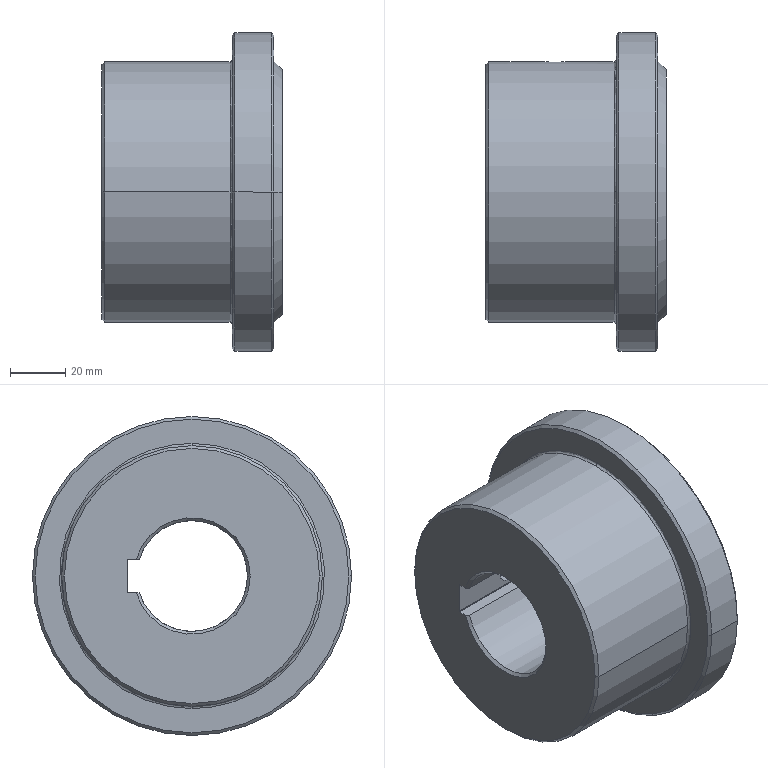Part | SolidWorks | features BaseBody 1 | 1 solid | 29 faces | box 65 x 115 x 115 mm | volume 415156 mm3 | cone 11 | cylinder 9 | plane 7 | spline 2 | commonest cylinder face diameters 0.5 x2 8.376 x2 94 x2 115 x2 40 x1